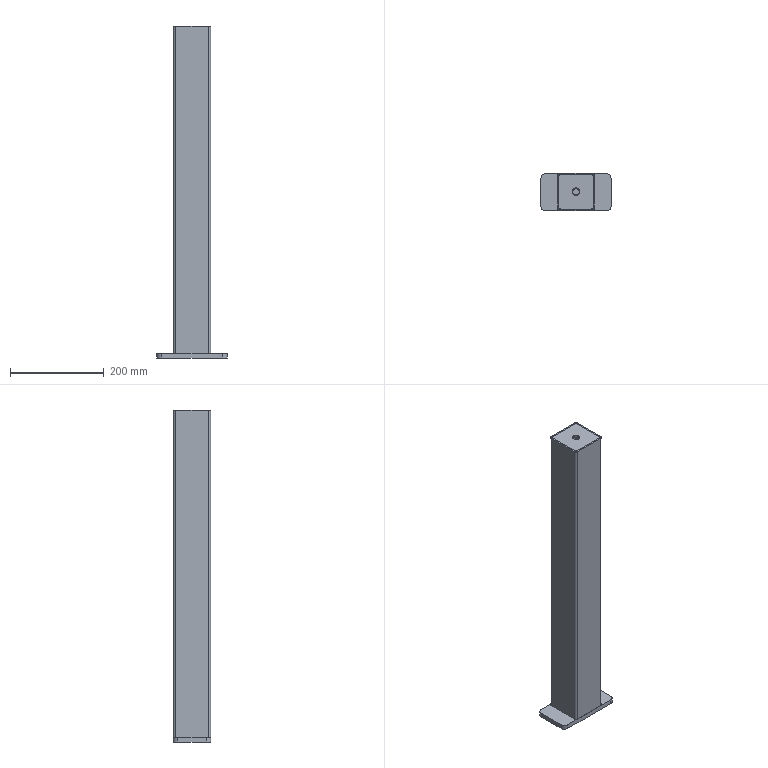Part | STEP file | 3 solids | 42 faces | box 150 x 80 x 710 mm | volume 779802 mm3 | plane 22 | cylinder 18 | cone 2 | commonest cylinder face diameters 10 x8 4 x4 20 x4 14 x2